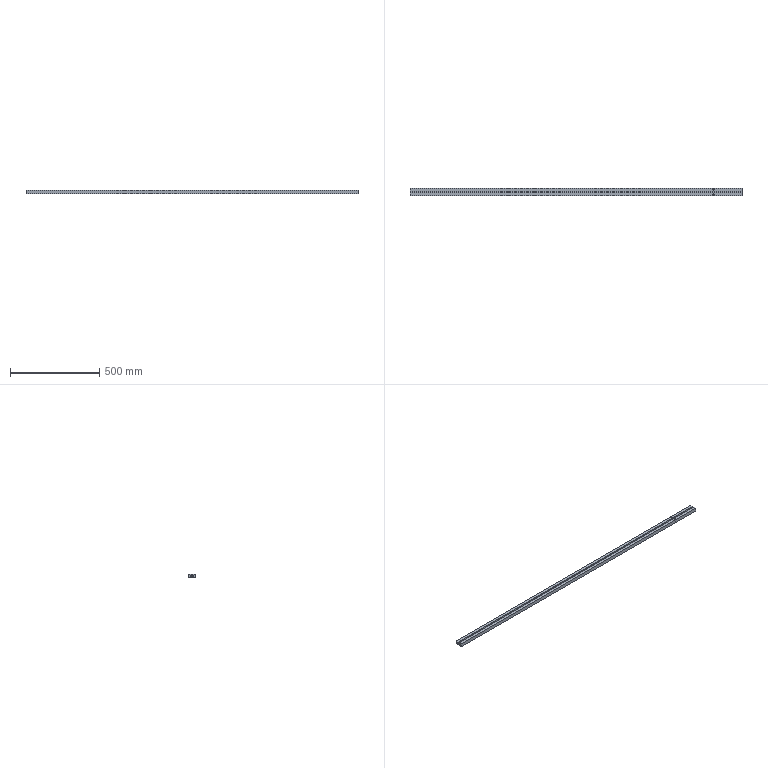Part | STEP file | DAOLIECHAO_1-2 | 1 solid | 28 faces | box 1861 x 40 x 20 mm | volume 1235153 mm3 | plane 20 | cylinder 8 | commonest cylinder face diameters 4.5 x4 8 x4
STEP:
#1=CARTESIAN_POINT('',(-377.75,-14.,-10.));
#2=VERTEX_POINT('',#1);
#3=CARTESIAN_POINT('',(-382.25,-14.,-10.));
#4=VERTEX_POINT('',#3);
#5=CARTESIAN_POINT('',(-380.,-14.,-10.));
#6=DIRECTION('',(0.,0.,-1.));
#7=DIRECTION('',(1.,0.,0.));
#8=AXIS2_PLACEMENT_3D('',#5,#6,#7);
#9=CIRCLE('',#8,2.25);
#10=EDGE_CURVE('',#2,#4,#9,.T.);
#11=ORIENTED_EDGE('',*,*,#10,.T.);
#12=CARTESIAN_POINT('',(-382.25,-14.,0.));
#13=VERTEX_POINT('',#12);
#14=CARTESIAN_POINT('',(-382.25,-14.,10.));
#15=DIRECTION('',(0.,0.,1.));
#16=VECTOR('',#15,1000.);
#17=LINE('',#14,#16);
#18=EDGE_CURVE('',#4,#13,#17,.T.);
#19=ORIENTED_EDGE('',*,*,#18,.T.);
#20=CARTESIAN_POINT('',(-377.75,-14.,0.));
#21=VERTEX_POINT('',#20);
#22=CARTESIAN_POINT('',(-380.,-14.,0.));
#23=DIRECTION('',(0.,0.,-1.));
#24=DIRECTION('',(1.,0.,0.));
#25=AXIS2_PLACEMENT_3D('',#22,#23,#24);
#26=CIRCLE('',#25,2.25);
#27=EDGE_CURVE('',#21,#13,#26,.T.);
#28=ORIENTED_EDGE('',*,*,#27,.F.);
#29=CARTESIAN_POINT('',(-377.75,-14.,10.));
#30=DIRECTION('',(0.,0.,1.));
#31=VECTOR('',#30,1000.);
#32=LINE('',#29,#31);
#33=EDGE_CURVE('',#2,#21,#32,.T.);
#34=ORIENTED_EDGE('',*,*,#33,.F.);
#35=EDGE_LOOP('',(#11,#19,#28,#34));
#36=FACE_OUTER_BOUND('',#35,.T.);
#37=CARTESIAN_POINT('',(-380.,-14.,10.));
#38=DIRECTION('',(0.,0.,1.));
#39=DIRECTION('',(1.,0.,0.));
#40=AXIS2_PLACEMENT_3D('',#37,#38,#39);
#41=CYLINDRICAL_SURFACE('',#40,2.25);
#42=ADVANCED_FACE('',(#36),#41,.F.);
#43=CARTESIAN_POINT('',(-377.75,14.,-10.));
#44=VERTEX_POINT('',#43);
#45=CARTESIAN_POINT('',(-382.25,14.,-10.));
#46=VERTEX_POINT('',#45);
#47=CARTESIAN_POINT('',(-380.,14.,-10.));
#48=DIRECTION('',(0.,0.,-1.));
#49=DIRECTION('',(1.,0.,0.));
#50=AXIS2_PLACEMENT_3D('',#47,#48,#49);
#51=CIRCLE('',#50,2.25);
#52=EDGE_CURVE('',#44,#46,#51,.T.);
#53=ORIENTED_EDGE('',*,*,#52,.T.);
#54=CARTESIAN_POINT('',(-382.25,14.,0.));
#55=VERTEX_POINT('',#54);
#56=CARTESIAN_POINT('',(-382.25,14.,10.));
#57=DIRECTION('',(0.,0.,1.));
#58=VECTOR('',#57,1000.);
#59=LINE('',#56,#58);
#60=EDGE_CURVE('',#46,#55,#59,.T.);
#61=ORIENTED_EDGE('',*,*,#60,.T.);
#62=CARTESIAN_POINT('',(-377.75,14.,0.));
#63=VERTEX_POINT('',#62);
#64=CARTESIAN_POINT('',(-380.,14.,0.));
#65=DIRECTION('',(0.,0.,-1.));
#66=DIRECTION('',(1.,0.,0.));
#67=AXIS2_PLACEMENT_3D('',#64,#65,#66);
#68=CIRCLE('',#67,2.25);
#69=EDGE_CURVE('',#63,#55,#68,.T.);
#70=ORIENTED_EDGE('',*,*,#69,.F.);
#71=CARTESIAN_POINT('',(-377.75,14.,10.));
#72=DIRECTION('',(0.,0.,1.));
#73=VECTOR('',#72,1000.);
#74=LINE('',#71,#73);
#75=EDGE_CURVE('',#44,#63,#74,.T.);
#76=ORIENTED_EDGE('',*,*,#75,.F.);
#77=EDGE_LOOP('',(#53,#61,#70,#76));
#78=FACE_OUTER_BOUND('',#77,.T.);
#79=CARTESIAN_POINT('',(-380.,14.,10.));
#80=DIRECTION('',(0.,0.,1.));
#81=DIRECTION('',(1.,0.,0.));
#82=AXIS2_PLACEMENT_3D('',#79,#80,#81);
#83=CYLINDRICAL_SURFACE('',#82,2.25);
#84=ADVANCED_FACE('',(#78),#83,.F.);
#85=CARTESIAN_POINT('',(-376.,-14.,0.));
#86=VERTEX_POINT('',#85);
#87=CARTESIAN_POINT('',(-384.,-14.,0.));
#88=VERTEX_POINT('',#87);
#89=CARTESIAN_POINT('',(-380.,-14.,0.));
#90=DIRECTION('',(0.,0.,-1.));
#91=DIRECTION('',(1.,0.,0.));
#92=AXIS2_PLACEMENT_3D('',#89,#90,#91);
#93=CIRCLE('',#92,4.);
#94=EDGE_CURVE('',#86,#88,#93,.T.);
#95=ORIENTED_EDGE('',*,*,#94,.T.);
#96=CARTESIAN_POINT('',(-384.,-14.,10.));
#97=VERTEX_POINT('',#96);
#98=CARTESIAN_POINT('',(-384.,-14.,10.));
#99=DIRECTION('',(0.,0.,1.));
#100=VECTOR('',#99,1000.);
#101=LINE('',#98,#100);
#102=EDGE_CURVE('',#88,#97,#101,.T.);
#103=ORIENTED_EDGE('',*,*,#102,.T.);
#104=CARTESIAN_POINT('',(-376.,-14.,10.));
#105=VERTEX_POINT('',#104);
#106=CARTESIAN_POINT('',(-380.,-14.,10.));
#107=DIRECTION('',(0.,0.,1.));
#108=DIRECTION('',(1.,0.,0.));
#109=AXIS2_PLACEMENT_3D('',#106,#107,#108);
#110=CIRCLE('',#109,4.);
#111=EDGE_CURVE('',#97,#105,#110,.T.);
#112=ORIENTED_EDGE('',*,*,#111,.T.);
#113=CARTESIAN_POINT('',(-376.,-14.,10.));
#114=DIRECTION('',(0.,0.,1.));
#115=VECTOR('',#114,1000.);
#116=LINE('',#113,#115);
#117=EDGE_CURVE('',#86,#105,#116,.T.);
#118=ORIENTED_EDGE('',*,*,#117,.F.);
#119=EDGE_LOOP('',(#95,#103,#112,#118));
#120=FACE_OUTER_BOUND('',#119,.T.);
#121=CARTESIAN_POINT('',(-380.,-14.,10.));
#122=DIRECTION('',(0.,0.,1.));
#123=DIRECTION('',(1.,0.,0.));
#124=AXIS2_PLACEMENT_3D('',#121,#122,#123);
#125=CYLINDRICAL_SURFACE('',#124,4.);
#126=ADVANCED_FACE('',(#120),#125,.F.);
#127=CARTESIAN_POINT('',(-376.,14.,0.));
#128=VERTEX_POINT('',#127);
#129=CARTESIAN_POINT('',(-384.,14.,0.));
#130=VERTEX_POINT('',#129);
#131=CARTESIAN_POINT('',(-380.,14.,0.));
#132=DIRECTION('',(0.,0.,-1.));
#133=DIRECTION('',(1.,0.,0.));
#134=AXIS2_PLACEMENT_3D('',#131,#132,#133);
#135=CIRCLE('',#134,4.);
#136=EDGE_CURVE('',#128,#130,#135,.T.);
#137=ORIENTED_EDGE('',*,*,#136,.T.);
#138=CARTESIAN_POINT('',(-384.,14.,10.));
#139=VERTEX_POINT('',#138);
#140=CARTESIAN_POINT('',(-384.,14.,10.));
#141=DIRECTION('',(0.,0.,1.));
#142=VECTOR('',#141,1000.);
#143=LINE('',#140,#142);
#144=EDGE_CURVE('',#130,#139,#143,.T.);
#145=ORIENTED_EDGE('',*,*,#144,.T.);
#146=CARTESIAN_POINT('',(-376.,14.,10.));
#147=VERTEX_POINT('',#146);
#148=CARTESIAN_POINT('',(-380.,14.,10.));
#149=DIRECTION('',(0.,0.,1.));
#150=DIRECTION('',(1.,0.,0.));
#151=AXIS2_PLACEMENT_3D('',#148,#149,#150);
#152=CIRCLE('',#151,4.);
#153=EDGE_CURVE('',#139,#147,#152,.T.);
#154=ORIENTED_EDGE('',*,*,#153,.T.);
#155=CARTESIAN_POINT('',(-376.,14.,10.));
#156=DIRECTION('',(0.,0.,1.));
#157=VECTOR('',#156,1000.);
#158=LINE('',#155,#157);
#159=EDGE_CURVE('',#128,#147,#158,.T.);
#160=ORIENTED_EDGE('',*,*,#159,.F.);
#161=EDGE_LOOP('',(#137,#145,#154,#160));
#162=FACE_OUTER_BOUND('',#161,.T.);
#163=CARTESIAN_POINT('',(-380.,14.,10.));
#164=DIRECTION('',(0.,0.,1.));
#165=DIRECTION('',(1.,0.,0.));
#166=AXIS2_PLACEMENT_3D('',#163,#164,#165);
#167=CYLINDRICAL_SURFACE('',#166,4.);
#168=ADVANCED_FACE('',(#162),#167,.F.);
#169=ORIENTED_EDGE('',*,*,#10,.F.);
#170=CARTESIAN_POINT('',(-380.,-14.,-10.));
#171=DIRECTION('',(0.,0.,-1.));
#172=DIRECTION('',(1.,0.,0.));
#173=AXIS2_PLACEMENT_3D('',#170,#171,#172);
#174=CIRCLE('',#173,2.25);
#175=EDGE_CURVE('',#4,#2,#174,.T.);
#176=ORIENTED_EDGE('',*,*,#175,.F.);
#177=EDGE_LOOP('',(#169,#176));
#178=FACE_BOUND('',#177,.T.);
#179=ORIENTED_EDGE('',*,*,#52,.F.);
#180=CARTESIAN_POINT('',(-380.,14.,-10.));
#181=DIRECTION('',(0.,0.,-1.));
#182=DIRECTION('',(1.,0.,0.));
#183=AXIS2_PLACEMENT_3D('',#180,#181,#182);
#184=CIRCLE('',#183,2.25);
#185=EDGE_CURVE('',#46,#44,#184,.T.);
#186=ORIENTED_EDGE('',*,*,#185,.F.);
#187=EDGE_LOOP('',(#179,#186));
#188=FACE_BOUND('',#187,.T.);
#189=CARTESIAN_POINT('',(-2082.,-20.,-10.));
#190=VERTEX_POINT('',#189);
#191=CARTESIAN_POINT('',(-220.621,-20.,-10.));
#192=VERTEX_POINT('',#191);
#193=CARTESIAN_POINT('',(400.,-20.,-10.));
#194=DIRECTION('',(1.,0.,0.));
#195=VECTOR('',#194,1000.);
#196=LINE('',#193,#195);
#197=EDGE_CURVE('',#190,#192,#196,.T.);
#198=ORIENTED_EDGE('',*,*,#197,.F.);
#199=CARTESIAN_POINT('',(-2082.,20.,-10.));
#200=VERTEX_POINT('',#199);
#201=CARTESIAN_POINT('',(-2082.,-20.,-10.));
#202=DIRECTION('',(0.,1.,0.));
#203=VECTOR('',#202,1000.);
#204=LINE('',#201,#203);
#205=EDGE_CURVE('',#190,#200,#204,.T.);
#206=ORIENTED_EDGE('',*,*,#205,.T.);
#207=CARTESIAN_POINT('',(-220.621,20.,-10.));
#208=VERTEX_POINT('',#207);
#209=CARTESIAN_POINT('',(400.,20.,-10.));
#210=DIRECTION('',(-1.,0.,0.));
#211=VECTOR('',#210,1000.);
#212=LINE('',#209,#211);
#213=EDGE_CURVE('',#208,#200,#212,.T.);
#214=ORIENTED_EDGE('',*,*,#213,.F.);
#215=CARTESIAN_POINT('',(-220.621,-20.,-10.));
#216=DIRECTION('',(0.,1.,0.));
#217=VECTOR('',#216,1000.);
#218=LINE('',#215,#217);
#219=EDGE_CURVE('',#192,#208,#218,.T.);
#220=ORIENTED_EDGE('',*,*,#219,.F.);
#221=EDGE_LOOP('',(#198,#206,#214,#220));
#222=FACE_OUTER_BOUND('',#221,.T.);
#223=CARTESIAN_POINT('',(400.,-20.,-10.));
#224=DIRECTION('',(0.,0.,1.));
#225=DIRECTION('',(1.,0.,0.));
#226=AXIS2_PLACEMENT_3D('',#223,#224,#225);
#227=PLANE('',#226);
#228=ADVANCED_FACE('',(#178,#188,#222),#227,.F.);
#229=ORIENTED_EDGE('',*,*,#18,.F.);
#230=ORIENTED_EDGE('',*,*,#175,.T.);
#231=ORIENTED_EDGE('',*,*,#33,.T.);
#232=CARTESIAN_POINT('',(-380.,-14.,0.));
#233=DIRECTION('',(0.,0.,-1.));
#234=DIRECTION('',(1.,0.,0.));
#235=AXIS2_PLACEMENT_3D('',#232,#233,#234);
#236=CIRCLE('',#235,2.25);
#237=EDGE_CURVE('',#13,#21,#236,.T.);
#238=ORIENTED_EDGE('',*,*,#237,.F.);
#239=EDGE_LOOP('',(#229,#230,#231,#238));
#240=FACE_OUTER_BOUND('',#239,.T.);
#241=CARTESIAN_POINT('',(-380.,-14.,10.));
#242=DIRECTION('',(0.,0.,1.));
#243=DIRECTION('',(1.,0.,0.));
#244=AXIS2_PLACEMENT_3D('',#241,#242,#243);
#245=CYLINDRICAL_SURFACE('',#244,2.25);
#246=ADVANCED_FACE('',(#240),#245,.F.);
#247=ORIENTED_EDGE('',*,*,#60,.F.);
#248=ORIENTED_EDGE('',*,*,#185,.T.);
#249=ORIENTED_EDGE('',*,*,#75,.T.);
#250=CARTESIAN_POINT('',(-380.,14.,0.));
#251=DIRECTION('',(0.,0.,-1.));
#252=DIRECTION('',(1.,0.,0.));
#253=AXIS2_PLACEMENT_3D('',#250,#251,#252);
#254=CIRCLE('',#253,2.25);
#255=EDGE_CURVE('',#55,#63,#254,.T.);
#256=ORIENTED_EDGE('',*,*,#255,.F.);
#257=EDGE_LOOP('',(#247,#248,#249,#256));
#258=FACE_OUTER_BOUND('',#257,.T.);
#259=CARTESIAN_POINT('',(-380.,14.,10.));
#260=DIRECTION('',(0.,0.,1.));
#261=DIRECTION('',(1.,0.,0.));
#262=AXIS2_PLACEMENT_3D('',#259,#260,#261);
#263=CYLINDRICAL_SURFACE('',#262,2.25);
#264=ADVANCED_FACE('',(#258),#263,.F.);
#265=ORIENTED_EDGE('',*,*,#213,.T.);
#266=CARTESIAN_POINT('',(-2082.,20.,10.));
#267=VERTEX_POINT('',#266);
#268=CARTESIAN_POINT('',(-2082.,20.,-10.));
#269=DIRECTION('',(0.,0.,1.));
#270=VECTOR('',#269,1000.);
#271=LINE('',#268,#270);
#272=EDGE_CURVE('',#200,#267,#271,.T.);
#273=ORIENTED_EDGE('',*,*,#272,.T.);
#274=CARTESIAN_POINT('',(-220.621,20.,10.));
#275=VERTEX_POINT('',#274);
#276=CARTESIAN_POINT('',(400.,20.,10.));
#277=DIRECTION('',(-1.,0.,0.));
#278=VECTOR('',#277,1000.);
#279=LINE('',#276,#278);
#280=EDGE_CURVE('',#275,#267,#279,.T.);
#281=ORIENTED_EDGE('',*,*,#280,.F.);
#282=CARTESIAN_POINT('',(-220.621,20.,-10.));
#283=DIRECTION('',(0.,0.,-1.));
#284=VECTOR('',#283,1000.);
#285=LINE('',#282,#284);
#286=EDGE_CURVE('',#275,#208,#285,.T.);
#287=ORIENTED_EDGE('',*,*,#286,.T.);
#288=EDGE_LOOP('',(#265,#273,#281,#287));
#289=FACE_OUTER_BOUND('',#288,.T.);
#290=CARTESIAN_POINT('',(400.,20.,-10.));
#291=DIRECTION('',(0.,-1.,0.));
#292=DIRECTION('',(0.,0.,-1.));
#293=AXIS2_PLACEMENT_3D('',#290,#291,#292);
#294=PLANE('',#293);
#295=ADVANCED_FACE('',(#289),#294,.F.);
#296=CARTESIAN_POINT('',(-2082.,-20.,10.));
#297=VERTEX_POINT('',#296);
#298=CARTESIAN_POINT('',(-220.621,-20.,10.));
#299=VERTEX_POINT('',#298);
#300=CARTESIAN_POINT('',(400.,-20.,10.));
#301=DIRECTION('',(1.,0.,0.));
#302=VECTOR('',#301,1000.);
#303=LINE('',#300,#302);
#304=EDGE_CURVE('',#297,#299,#303,.T.);
#305=ORIENTED_EDGE('',*,*,#304,.F.);
#306=CARTESIAN_POINT('',(-2082.,-20.,-10.));
#307=DIRECTION('',(0.,0.,-1.));
#308=VECTOR('',#307,1000.);
#309=LINE('',#306,#308);
#310=EDGE_CURVE('',#297,#190,#309,.T.);
#311=ORIENTED_EDGE('',*,*,#310,.T.);
#312=ORIENTED_EDGE('',*,*,#197,.T.);
#313=CARTESIAN_POINT('',(-220.621,-20.,10.));
#314=DIRECTION('',(0.,0.,-1.));
#315=VECTOR('',#314,1000.);
#316=LINE('',#313,#315);
#317=EDGE_CURVE('',#299,#192,#316,.T.);
#318=ORIENTED_EDGE('',*,*,#317,.F.);
#319=EDGE_LOOP('',(#305,#311,#312,#318));
#320=FACE_OUTER_BOUND('',#319,.T.);
#321=CARTESIAN_POINT('',(400.,-20.,-10.));
#322=DIRECTION('',(0.,1.,0.));
#323=DIRECTION('',(0.,0.,1.));
#324=AXIS2_PLACEMENT_3D('',#321,#322,#323);
#325=PLANE('',#324);
#326=ADVANCED_FACE('',(#320),#325,.F.);
#327=ORIENTED_EDGE('',*,*,#27,.T.);
#328=ORIENTED_EDGE('',*,*,#237,.T.);
#329=EDGE_LOOP('',(#327,#328));
#330=FACE_BOUND('',#329,.T.);
#331=ORIENTED_EDGE('',*,*,#94,.F.);
#332=CARTESIAN_POINT('',(-380.,-14.,0.));
#333=DIRECTION('',(0.,0.,-1.));
#334=DIRECTION('',(1.,0.,0.));
#335=AXIS2_PLACEMENT_3D('',#332,#333,#334);
#336=CIRCLE('',#335,4.);
#337=EDGE_CURVE('',#88,#86,#336,.T.);
#338=ORIENTED_EDGE('',*,*,#337,.F.);
#339=EDGE_LOOP('',(#331,#338));
#340=FACE_OUTER_BOUND('',#339,.T.);
#341=CARTESIAN_POINT('',(-377.75,-14.,0.));
#342=DIRECTION('',(0.,0.,-1.));
#343=DIRECTION('',(-1.,0.,0.));
#344=AXIS2_PLACEMENT_3D('',#341,#342,#343);
#345=PLANE('',#344);
#346=ADVANCED_FACE('',(#330,#340),#345,.F.);
#347=ORIENTED_EDGE('',*,*,#69,.T.);
#348=ORIENTED_EDGE('',*,*,#255,.T.);
#349=EDGE_LOOP('',(#347,#348));
#350=FACE_BOUND('',#349,.T.);
#351=ORIENTED_EDGE('',*,*,#136,.F.);
#352=CARTESIAN_POINT('',(-380.,14.,0.));
#353=DIRECTION('',(0.,0.,-1.));
#354=DIRECTION('',(1.,0.,0.));
#355=AXIS2_PLACEMENT_3D('',#352,#353,#354);
#356=CIRCLE('',#355,4.);
#357=EDGE_CURVE('',#130,#128,#356,.T.);
#358=ORIENTED_EDGE('',*,*,#357,.F.);
#359=EDGE_LOOP('',(#351,#358));
#360=FACE_OUTER_BOUND('',#359,.T.);
#361=CARTESIAN_POINT('',(-377.75,14.,0.));
#362=DIRECTION('',(0.,0.,-1.));
#363=DIRECTION('',(-1.,0.,0.));
#364=AXIS2_PLACEMENT_3D('',#361,#362,#363);
#365=PLANE('',#364);
#366=ADVANCED_FACE('',(#350,#360),#365,.F.);
#367=CARTESIAN_POINT('',(-380.,14.,10.));
#368=DIRECTION('',(0.,0.,1.));
#369=DIRECTION('',(1.,0.,0.));
#370=AXIS2_PLACEMENT_3D('',#367,#368,#369);
#371=CIRCLE('',#370,4.);
#372=EDGE_CURVE('',#147,#139,#371,.T.);
#373=ORIENTED_EDGE('',*,*,#372,.F.);
#374=ORIENTED_EDGE('',*,*,#153,.F.);
#375=EDGE_LOOP('',(#373,#374));
#376=FACE_BOUND('',#375,.T.);
#377=ORIENTED_EDGE('',*,*,#280,.T.);
#378=CARTESIAN_POINT('',(-2082.,4.2,10.));
#379=VERTEX_POINT('',#378);
#380=CARTESIAN_POINT('',(-2082.,-22.,10.));
#381=DIRECTION('',(0.,1.,0.));
#382=VECTOR('',#381,1000.);
#383=LINE('',#380,#382);
#384=EDGE_CURVE('',#379,#267,#383,.T.);
#385=ORIENTED_EDGE('',*,*,#384,.F.);
#386=CARTESIAN_POINT('',(-220.621,4.2,10.));
#387=VERTEX_POINT('',#386);
#388=CARTESIAN_POINT('',(400.,4.2,10.));
#389=DIRECTION('',(-1.,0.,0.));
#390=VECTOR('',#389,1000.);
#391=LINE('',#388,#390);
#392=EDGE_CURVE('',#387,#379,#391,.T.);
#393=ORIENTED_EDGE('',*,*,#392,.F.);
#394=CARTESIAN_POINT('',(-220.621,-20.,10.));
#395=DIRECTION('',(0.,1.,0.));
#396=VECTOR('',#395,1000.);
#397=LINE('',#394,#396);
#398=EDGE_CURVE('',#387,#275,#397,.T.);
#399=ORIENTED_EDGE('',*,*,#398,.T.);
#400=EDGE_LOOP('',(#377,#385,#393,#399));
#401=FACE_OUTER_BOUND('',#400,.T.);
#402=CARTESIAN_POINT('',(400.,-20.,10.));
#403=DIRECTION('',(0.,0.,-1.));
#404=DIRECTION('',(-1.,0.,0.));
#405=AXIS2_PLACEMENT_3D('',#402,#403,#404);
#406=PLANE('',#405);
#407=ADVANCED_FACE('',(#376,#401),#406,.F.);
#408=ORIENTED_EDGE('',*,*,#392,.T.);
#409=CARTESIAN_POINT('',(-2082.,4.2,2.6));
#410=VERTEX_POINT('',#409);
#411=CARTESIAN_POINT('',(-2082.,4.2,10.));
#412=DIRECTION('',(0.,0.,-1.));
#413=VECTOR('',#412,1000.);
#414=LINE('',#411,#413);
#415=EDGE_CURVE('',#379,#410,#414,.T.);
#416=ORIENTED_EDGE('',*,*,#415,.T.);
#417=CARTESIAN_POINT('',(-220.621,4.2,2.6));
#418=VERTEX_POINT('',#417);
#419=CARTESIAN_POINT('',(-400.,4.2,2.6));
#420=DIRECTION('',(-1.,0.,0.));
#421=VECTOR('',#420,1000.);
#422=LINE('',#419,#421);
#423=EDGE_CURVE('',#418,#410,#422,.T.);
#424=ORIENTED_EDGE('',*,*,#423,.F.);
#425=CARTESIAN_POINT('',(-220.621,4.2,10.));
#426=DIRECTION('',(0.,0.,1.));
#427=VECTOR('',#426,1000.);
#428=LINE('',#425,#427);
#429=EDGE_CURVE('',#418,#387,#428,.T.);
#430=ORIENTED_EDGE('',*,*,#429,.T.);
#431=EDGE_LOOP('',(#408,#416,#424,#430));
#432=FACE_OUTER_BOUND('',#431,.T.);
#433=CARTESIAN_POINT('',(-400.,4.2,10.));
#434=DIRECTION('',(0.,1.,0.));
#435=DIRECTION('',(0.,0.,1.));
#436=AXIS2_PLACEMENT_3D('',#433,#434,#435);
#437=PLANE('',#436);
#438=ADVANCED_FACE('',(#432),#437,.F.);
#439=CARTESIAN_POINT('',(-380.,-14.,10.));
#440=DIRECTION('',(0.,0.,1.));
#441=DIRECTION('',(1.,0.,0.));
#442=AXIS2_PLACEMENT_3D('',#439,#440,#441);
#443=CIRCLE('',#442,4.);
#444=EDGE_CURVE('',#105,#97,#443,.T.);
#445=ORIENTED_EDGE('',*,*,#444,.F.);
#446=ORIENTED_EDGE('',*,*,#111,.F.);
#447=EDGE_LOOP('',(#445,#446));
#448=FACE_BOUND('',#447,.T.);
#449=CARTESIAN_POINT('',(-2082.,-4.2,10.));
#450=VERTEX_POINT('',#449);
#451=CARTESIAN_POINT('',(-220.621,-4.2,10.));
#452=VERTEX_POINT('',#451);
#453=CARTESIAN_POINT('',(400.,-4.2,10.));
#454=DIRECTION('',(1.,0.,0.));
#455=VECTOR('',#454,1000.);
#456=LINE('',#453,#455);
#457=EDGE_CURVE('',#450,#452,#456,.T.);
#458=ORIENTED_EDGE('',*,*,#457,.F.);
#459=CARTESIAN_POINT('',(-2082.,-22.,10.));
#460=DIRECTION('',(0.,1.,0.));
#461=VECTOR('',#460,1000.);
#462=LINE('',#459,#461);
#463=EDGE_CURVE('',#297,#450,#462,.T.);
#464=ORIENTED_EDGE('',*,*,#463,.F.);
#465=ORIENTED_EDGE('',*,*,#304,.T.);
#466=CARTESIAN_POINT('',(-220.621,-20.,10.));
#467=DIRECTION('',(0.,1.,0.));
#468=VECTOR('',#467,1000.);
#469=LINE('',#466,#468);
#470=EDGE_CURVE('',#299,#452,#469,.T.);
#471=ORIENTED_EDGE('',*,*,#470,.T.);
#472=EDGE_LOOP('',(#458,#464,#465,#471));
#473=FACE_OUTER_BOUND('',#472,.T.);
#474=CARTESIAN_POINT('',(400.,-20.,10.));
#475=DIRECTION('',(0.,0.,-1.));
#476=DIRECTION('',(-1.,0.,0.));
#477=AXIS2_PLACEMENT_3D('',#474,#475,#476);
#478=PLANE('',#477);
#479=ADVANCED_FACE('',(#448,#473),#478,.F.);
#480=CARTESIAN_POINT('',(-2082.,-4.2,2.6));
#481=VERTEX_POINT('',#480);
#482=CARTESIAN_POINT('',(-220.621,-4.2,2.6));
#483=VERTEX_POINT('',#482);
#484=CARTESIAN_POINT('',(-400.,-4.2,2.6));
#485=DIRECTION('',(1.,0.,0.));
#486=VECTOR('',#485,1000.);
#487=LINE('',#484,#486);
#488=EDGE_CURVE('',#481,#483,#487,.T.);
#489=ORIENTED_EDGE('',*,*,#488,.F.);
#490=CARTESIAN_POINT('',(-2082.,-4.2,2.6));
#491=DIRECTION('',(0.,0.,1.));
#492=VECTOR('',#491,1000.);
#493=LINE('',#490,#492);
#494=EDGE_CURVE('',#481,#450,#493,.T.);
#495=ORIENTED_EDGE('',*,*,#494,.T.);
#496=ORIENTED_EDGE('',*,*,#457,.T.);
#497=CARTESIAN_POINT('',(-220.621,-4.2,2.6));
#498=DIRECTION('',(0.,0.,-1.));
#499=VECTOR('',#498,1000.);
#500=LINE('',#497,#499);
#501=EDGE_CURVE('',#452,#483,#500,.T.);
#502=ORIENTED_EDGE('',*,*,#501,.T.);
#503=EDGE_LOOP('',(#489,#495,#496,#502));
#504=FACE_OUTER_BOUND('',#503,.T.);
#505=CARTESIAN_POINT('',(-400.,-4.2,2.6));
#506=DIRECTION('',(0.,-1.,0.));
#507=DIRECTION('',(0.,0.,-1.));
#508=AXIS2_PLACEMENT_3D('',#505,#506,#507);
#509=PLANE('',#508);
#510=ADVANCED_FACE('',(#504),#509,.F.);
#511=CARTESIAN_POINT('',(-2082.,-6.6,2.6));
#512=VERTEX_POINT('',#511);
#513=CARTESIAN_POINT('',(-220.621,-6.6,2.6));
#514=VERTEX_POINT('',#513);
#515=CARTESIAN_POINT('',(-400.,-6.6,2.6));
#516=DIRECTION('',(1.,0.,0.));
#517=VECTOR('',#516,1000.);
#518=LINE('',#515,#517);
#519=EDGE_CURVE('',#512,#514,#518,.T.);
#520=ORIENTED_EDGE('',*,*,#519,.F.);
#521=CARTESIAN_POINT('',(-2082.,-6.6,2.6));
#522=DIRECTION('',(0.,1.,0.));
#523=VECTOR('',#522,1000.);
#524=LINE('',#521,#523);
#525=EDGE_CURVE('',#512,#481,#524,.T.);
#526=ORIENTED_EDGE('',*,*,#525,.T.);
#527=ORIENTED_EDGE('',*,*,#488,.T.);
#528=CARTESIAN_POINT('',(-220.621,-6.6,2.6));
#529=DIRECTION('',(0.,-1.,0.));
#530=VECTOR('',#529,1000.);
#531=LINE('',#528,#530);
#532=EDGE_CURVE('',#483,#514,#531,.T.);
#533=ORIENTED_EDGE('',*,*,#532,.T.);
#534=EDGE_LOOP('',(#520,#526,#527,#533));
#535=FACE_OUTER_BOUND('',#534,.T.);
#536=CARTESIAN_POINT('',(-400.,-6.6,2.6));
#537=DIRECTION('',(0.,0.,1.));
#538=DIRECTION('',(1.,0.,0.));
#539=AXIS2_PLACEMENT_3D('',#536,#537,#538);
#540=PLANE('',#539);
#541=ADVANCED_FACE('',(#535),#540,.F.);
#542=CARTESIAN_POINT('',(-2082.,-6.6,-1.7));
#543=VERTEX_POINT('',#542);
#544=CARTESIAN_POINT('',(-220.621,-6.6,-1.7));
#545=VERTEX_POINT('',#544);
#546=CARTESIAN_POINT('',(-400.,-6.6,-1.7));
#547=DIRECTION('',(1.,0.,0.));
#548=VECTOR('',#547,1000.);
#549=LINE('',#546,#548);
#550=EDGE_CURVE('',#543,#545,#549,.T.);
#551=ORIENTED_EDGE('',*,*,#550,.F.);
#552=CARTESIAN_POINT('',(-2082.,-6.6,-1.7));
#553=DIRECTION('',(0.,0.,1.));
#554=VECTOR('',#553,1000.);
#555=LINE('',#552,#554);
#556=EDGE_CURVE('',#543,#512,#555,.T.);
#557=ORIENTED_EDGE('',*,*,#556,.T.);
#558=ORIENTED_EDGE('',*,*,#519,.T.);
#559=CARTESIAN_POINT('',(-220.621,-6.6,-1.7));
#560=DIRECTION('',(0.,0.,-1.));
#561=VECTOR('',#560,1000.);
#562=LINE('',#559,#561);
#563=EDGE_CURVE('',#514,#545,#562,.T.);
#564=ORIENTED_EDGE('',*,*,#563,.T.);
#565=EDGE_LOOP('',(#551,#557,#558,#564));
#566=FACE_OUTER_BOUND('',#565,.T.);
#567=CARTESIAN_POINT('',(-400.,-6.6,-1.7));
#568=DIRECTION('',(0.,-1.,0.));
#569=DIRECTION('',(0.,0.,-1.));
#570=AXIS2_PLACEMENT_3D('',#567,#568,#569);
#571=PLANE('',#570);
#572=ADVANCED_FACE('',(#566),#571,.F.);
#573=CARTESIAN_POINT('',(-2082.,-4.2,-1.7));
#574=VERTEX_POINT('',#573);
#575=CARTESIAN_POINT('',(-220.621,-4.2,-1.7));
#576=VERTEX_POINT('',#575);
#577=CARTESIAN_POINT('',(-400.,-4.2,-1.7));
#578=DIRECTION('',(1.,0.,0.));
#579=VECTOR('',#578,1000.);
#580=LINE('',#577,#579);
#581=EDGE_CURVE('',#574,#576,#580,.T.);
#582=ORIENTED_EDGE('',*,*,#581,.F.);
#583=CARTESIAN_POINT('',(-2082.,-4.2,-1.7));
#584=DIRECTION('',(0.,-1.,0.));
#585=VECTOR('',#584,1000.);
#586=LINE('',#583,#585);
#587=EDGE_CURVE('',#574,#543,#586,.T.);
#588=ORIENTED_EDGE('',*,*,#587,.T.);
#589=ORIENTED_EDGE('',*,*,#550,.T.);
#590=CARTESIAN_POINT('',(-220.621,-4.2,-1.7));
#591=DIRECTION('',(0.,1.,0.));
#592=VECTOR('',#591,1000.);
#593=LINE('',#590,#592);
#594=EDGE_CURVE('',#545,#576,#593,.T.);
#595=ORIENTED_EDGE('',*,*,#594,.T.);
#596=EDGE_LOOP('',(#582,#588,#589,#595));
#597=FACE_OUTER_BOUND('',#596,.T.);
#598=CARTESIAN_POINT('',(-400.,-4.2,-1.7));
#599=DIRECTION('',(0.,0.,-1.));
#600=DIRECTION('',(-1.,0.,0.));
#601=AXIS2_PLACEMENT_3D('',#598,#599,#600);
#602=PLANE('',#601);
#603=ADVANCED_FACE('',(#597),#602,.F.);
#604=CARTESIAN_POINT('',(-2082.,-4.2,-3.7));
#605=VERTEX_POINT('',#604);
#606=CARTESIAN_POINT('',(-220.621,-4.2,-3.7));
#607=VERTEX_POINT('',#606);
#608=CARTESIAN_POINT('',(-400.,-4.2,-3.7));
#609=DIRECTION('',(1.,0.,0.));
#610=VECTOR('',#609,1000.);
#611=LINE('',#608,#610);
#612=EDGE_CURVE('',#605,#607,#611,.T.);
#613=ORIENTED_EDGE('',*,*,#612,.F.);
#614=CARTESIAN_POINT('',(-2082.,-4.2,-3.7));
#615=DIRECTION('',(0.,0.,1.));
#616=VECTOR('',#615,1000.);
#617=LINE('',#614,#616);
#618=EDGE_CURVE('',#605,#574,#617,.T.);
#619=ORIENTED_EDGE('',*,*,#618,.T.);
#620=ORIENTED_EDGE('',*,*,#581,.T.);
#621=CARTESIAN_POINT('',(-220.621,-4.2,-3.7));
#622=DIRECTION('',(0.,0.,-1.));
#623=VECTOR('',#622,1000.);
#624=LINE('',#621,#623);
#625=EDGE_CURVE('',#576,#607,#624,.T.);
#626=ORIENTED_EDGE('',*,*,#625,.T.);
#627=EDGE_LOOP('',(#613,#619,#620,#626));
#628=FACE_OUTER_BOUND('',#627,.T.);
#629=CARTESIAN_POINT('',(-400.,-4.2,-3.7));
#630=DIRECTION('',(0.,-1.,0.));
#631=DIRECTION('',(0.,0.,-1.));
#632=AXIS2_PLACEMENT_3D('',#629,#630,#631);
#633=PLANE('',#632);
#634=ADVANCED_FACE('',(#628),#633,.F.);
#635=CARTESIAN_POINT('',(-2082.,4.2,-3.7));
#636=VERTEX_POINT('',#635);
#637=CARTESIAN_POINT('',(-220.621,4.2,-3.7));
#638=VERTEX_POINT('',#637);
#639=CARTESIAN_POINT('',(-400.,4.2,-3.7));
#640=DIRECTION('',(1.,0.,0.));
#641=VECTOR('',#640,1000.);
#642=LINE('',#639,#641);
#643=EDGE_CURVE('',#636,#638,#642,.T.);
#644=ORIENTED_EDGE('',*,*,#643,.F.);
#645=CARTESIAN_POINT('',(-2082.,4.2,-3.7));
#646=DIRECTION('',(0.,-1.,0.));
#647=VECTOR('',#646,1000.);
#648=LINE('',#645,#647);
#649=EDGE_CURVE('',#636,#605,#648,.T.);
#650=ORIENTED_EDGE('',*,*,#649,.T.);
#651=ORIENTED_EDGE('',*,*,#612,.T.);
#652=CARTESIAN_POINT('',(-220.621,4.2,-3.7));
#653=DIRECTION('',(0.,1.,0.));
#654=VECTOR('',#653,1000.);
#655=LINE('',#652,#654);
#656=EDGE_CURVE('',#607,#638,#655,.T.);
#657=ORIENTED_EDGE('',*,*,#656,.T.);
#658=EDGE_LOOP('',(#644,#650,#651,#657));
#659=FACE_OUTER_BOUND('',#658,.T.);
#660=CARTESIAN_POINT('',(-400.,4.2,-3.7));
#661=DIRECTION('',(0.,0.,-1.));
#662=DIRECTION('',(-1.,0.,0.));
#663=AXIS2_PLACEMENT_3D('',#660,#661,#662);
#664=PLANE('',#663);
#665=ADVANCED_FACE('',(#659),#664,.F.);
#666=CARTESIAN_POINT('',(-2082.,4.2,-1.7));
#667=VERTEX_POINT('',#666);
#668=CARTESIAN_POINT('',(-220.621,4.2,-1.7));
#669=VERTEX_POINT('',#668);
#670=CARTESIAN_POINT('',(-400.,4.2,-1.7));
#671=DIRECTION('',(1.,0.,0.));
#672=VECTOR('',#671,1000.);
#673=LINE('',#670,#672);
#674=EDGE_CURVE('',#667,#669,#673,.T.);
#675=ORIENTED_EDGE('',*,*,#674,.F.);
#676=CARTESIAN_POINT('',(-2082.,4.2,-1.7));
#677=DIRECTION('',(0.,0.,-1.));
#678=VECTOR('',#677,1000.);
#679=LINE('',#676,#678);
#680=EDGE_CURVE('',#667,#636,#679,.T.);
#681=ORIENTED_EDGE('',*,*,#680,.T.);
#682=ORIENTED_EDGE('',*,*,#643,.T.);
#683=CARTESIAN_POINT('',(-220.621,4.2,-1.7));
#684=DIRECTION('',(0.,0.,1.));
#685=VECTOR('',#684,1000.);
#686=LINE('',#683,#685);
#687=EDGE_CURVE('',#638,#669,#686,.T.);
#688=ORIENTED_EDGE('',*,*,#687,.T.);
#689=EDGE_LOOP('',(#675,#681,#682,#688));
#690=FACE_OUTER_BOUND('',#689,.T.);
#691=CARTESIAN_POINT('',(-400.,4.2,-1.7));
#692=DIRECTION('',(0.,1.,0.));
#693=DIRECTION('',(0.,0.,1.));
#694=AXIS2_PLACEMENT_3D('',#691,#692,#693);
#695=PLANE('',#694);
#696=ADVANCED_FACE('',(#690),#695,.F.);
#697=CARTESIAN_POINT('',(-2082.,6.6,-1.7));
#698=VERTEX_POINT('',#697);
#699=CARTESIAN_POINT('',(-220.621,6.6,-1.7));
#700=VERTEX_POINT('',#699);
#701=CARTESIAN_POINT('',(-400.,6.6,-1.7));
#702=DIRECTION('',(1.,0.,0.));
#703=VECTOR('',#702,1000.);
#704=LINE('',#701,#703);
#705=EDGE_CURVE('',#698,#700,#704,.T.);
#706=ORIENTED_EDGE('',*,*,#705,.F.);
#707=CARTESIAN_POINT('',(-2082.,6.6,-1.7));
#708=DIRECTION('',(0.,-1.,0.));
#709=VECTOR('',#708,1000.);
#710=LINE('',#707,#709);
#711=EDGE_CURVE('',#698,#667,#710,.T.);
#712=ORIENTED_EDGE('',*,*,#711,.T.);
#713=ORIENTED_EDGE('',*,*,#674,.T.);
#714=CARTESIAN_POINT('',(-220.621,6.6,-1.7));
#715=DIRECTION('',(0.,1.,0.));
#716=VECTOR('',#715,1000.);
#717=LINE('',#714,#716);
#718=EDGE_CURVE('',#669,#700,#717,.T.);
#719=ORIENTED_EDGE('',*,*,#718,.T.);
#720=EDGE_LOOP('',(#706,#712,#713,#719));
#721=FACE_OUTER_BOUND('',#720,.T.);
#722=CARTESIAN_POINT('',(-400.,6.6,-1.7));
#723=DIRECTION('',(0.,0.,-1.));
#724=DIRECTION('',(-1.,0.,0.));
#725=AXIS2_PLACEMENT_3D('',#722,#723,#724);
#726=PLANE('',#725);
#727=ADVANCED_FACE('',(#721),#726,.F.);
#728=CARTESIAN_POINT('',(-2082.,6.6,2.6));
#729=VERTEX_POINT('',#728);
#730=CARTESIAN_POINT('',(-220.621,6.6,2.6));
#731=VERTEX_POINT('',#730);
#732=CARTESIAN_POINT('',(-400.,6.6,2.6));
#733=DIRECTION('',(1.,0.,0.));
#734=VECTOR('',#733,1000.);
#735=LINE('',#732,#734);
#736=EDGE_CURVE('',#729,#731,#735,.T.);
#737=ORIENTED_EDGE('',*,*,#736,.F.);
#738=CARTESIAN_POINT('',(-2082.,6.6,2.6));
#739=DIRECTION('',(0.,0.,-1.));
#740=VECTOR('',#739,1000.);
#741=LINE('',#738,#740);
#742=EDGE_CURVE('',#729,#698,#741,.T.);
#743=ORIENTED_EDGE('',*,*,#742,.T.);
#744=ORIENTED_EDGE('',*,*,#705,.T.);
#745=CARTESIAN_POINT('',(-220.621,6.6,2.6));
#746=DIRECTION('',(0.,0.,1.));
#747=VECTOR('',#746,1000.);
#748=LINE('',#745,#747);
#749=EDGE_CURVE('',#700,#731,#748,.T.);
#750=ORIENTED_EDGE('',*,*,#749,.T.);
#751=EDGE_LOOP('',(#737,#743,#744,#750));
#752=FACE_OUTER_BOUND('',#751,.T.);
#753=CARTESIAN_POINT('',(-400.,6.6,2.6));
#754=DIRECTION('',(0.,1.,0.));
#755=DIRECTION('',(0.,0.,1.));
#756=AXIS2_PLACEMENT_3D('',#753,#754,#755);
#757=PLANE('',#756);
#758=ADVANCED_FACE('',(#752),#757,.F.);
#759=ORIENTED_EDGE('',*,*,#423,.T.);
#760=CARTESIAN_POINT('',(-2082.,4.2,2.6));
#761=DIRECTION('',(0.,1.,0.));
#762=VECTOR('',#761,1000.);
#763=LINE('',#760,#762);
#764=EDGE_CURVE('',#410,#729,#763,.T.);
#765=ORIENTED_EDGE('',*,*,#764,.T.);
#766=ORIENTED_EDGE('',*,*,#736,.T.);
#767=CARTESIAN_POINT('',(-220.621,4.2,2.6));
#768=DIRECTION('',(0.,-1.,0.));
#769=VECTOR('',#768,1000.);
#770=LINE('',#767,#769);
#771=EDGE_CURVE('',#731,#418,#770,.T.);
#772=ORIENTED_EDGE('',*,*,#771,.T.);
#773=EDGE_LOOP('',(#759,#765,#766,#772));
#774=FACE_OUTER_BOUND('',#773,.T.);
#775=CARTESIAN_POINT('',(-400.,4.2,2.6));
#776=DIRECTION('',(0.,0.,1.));
#777=DIRECTION('',(1.,0.,0.));
#778=AXIS2_PLACEMENT_3D('',#775,#776,#777);
#779=PLANE('',#778);
#780=ADVANCED_FACE('',(#774),#779,.F.);
#781=ORIENTED_EDGE('',*,*,#102,.F.);
#782=ORIENTED_EDGE('',*,*,#337,.T.);
#783=ORIENTED_EDGE('',*,*,#117,.T.);
#784=ORIENTED_EDGE('',*,*,#444,.T.);
#785=EDGE_LOOP('',(#781,#782,#783,#784));
#786=FACE_OUTER_BOUND('',#785,.T.);
#787=CARTESIAN_POINT('',(-380.,-14.,10.));
#788=DIRECTION('',(0.,0.,1.));
#789=DIRECTION('',(1.,0.,0.));
#790=AXIS2_PLACEMENT_3D('',#787,#788,#789);
#791=CYLINDRICAL_SURFACE('',#790,4.);
#792=ADVANCED_FACE('',(#786),#791,.F.);
#793=ORIENTED_EDGE('',*,*,#144,.F.);
#794=ORIENTED_EDGE('',*,*,#357,.T.);
#795=ORIENTED_EDGE('',*,*,#159,.T.);
#796=ORIENTED_EDGE('',*,*,#372,.T.);
#797=EDGE_LOOP('',(#793,#794,#795,#796));
#798=FACE_OUTER_BOUND('',#797,.T.);
#799=CARTESIAN_POINT('',(-380.,14.,10.));
#800=DIRECTION('',(0.,0.,1.));
#801=DIRECTION('',(1.,0.,0.));
#802=AXIS2_PLACEMENT_3D('',#799,#800,#801);
#803=CYLINDRICAL_SURFACE('',#802,4.);
#804=ADVANCED_FACE('',(#798),#803,.F.);
#805=ORIENTED_EDGE('',*,*,#470,.F.);
#806=ORIENTED_EDGE('',*,*,#317,.T.);
#807=ORIENTED_EDGE('',*,*,#219,.T.);
#808=ORIENTED_EDGE('',*,*,#286,.F.);
#809=ORIENTED_EDGE('',*,*,#398,.F.);
#810=ORIENTED_EDGE('',*,*,#429,.F.);
#811=ORIENTED_EDGE('',*,*,#771,.F.);
#812=ORIENTED_EDGE('',*,*,#749,.F.);
#813=ORIENTED_EDGE('',*,*,#718,.F.);
#814=ORIENTED_EDGE('',*,*,#687,.F.);
#815=ORIENTED_EDGE('',*,*,#656,.F.);
#816=ORIENTED_EDGE('',*,*,#625,.F.);
#817=ORIENTED_EDGE('',*,*,#594,.F.);
#818=ORIENTED_EDGE('',*,*,#563,.F.);
#819=ORIENTED_EDGE('',*,*,#532,.F.);
#820=ORIENTED_EDGE('',*,*,#501,.F.);
#821=EDGE_LOOP('',(#805,#806,#807,#808,#809,#810,#811,#812,#813,#814,#815,#816,#817,#818,#819,#820));
#822=FACE_OUTER_BOUND('',#821,.T.);
#823=CARTESIAN_POINT('',(-220.621,-20.,10.));
#824=DIRECTION('',(-1.,0.,0.));
#825=DIRECTION('',(0.,0.,1.));
#826=AXIS2_PLACEMENT_3D('',#823,#824,#825);
#827=PLANE('',#826);
#828=ADVANCED_FACE('',(#822),#827,.F.);
#829=ORIENTED_EDGE('',*,*,#525,.F.);
#830=ORIENTED_EDGE('',*,*,#556,.F.);
#831=ORIENTED_EDGE('',*,*,#587,.F.);
#832=ORIENTED_EDGE('',*,*,#618,.F.);
#833=ORIENTED_EDGE('',*,*,#649,.F.);
#834=ORIENTED_EDGE('',*,*,#680,.F.);
#835=ORIENTED_EDGE('',*,*,#711,.F.);
#836=ORIENTED_EDGE('',*,*,#742,.F.);
#837=ORIENTED_EDGE('',*,*,#764,.F.);
#838=ORIENTED_EDGE('',*,*,#415,.F.);
#839=ORIENTED_EDGE('',*,*,#384,.T.);
#840=ORIENTED_EDGE('',*,*,#272,.F.);
#841=ORIENTED_EDGE('',*,*,#205,.F.);
#842=ORIENTED_EDGE('',*,*,#310,.F.);
#843=ORIENTED_EDGE('',*,*,#463,.T.);
#844=ORIENTED_EDGE('',*,*,#494,.F.);
#845=EDGE_LOOP('',(#829,#830,#831,#832,#833,#834,#835,#836,#837,#838,#839,#840,#841,#842,#843,#844));
#846=FACE_OUTER_BOUND('',#845,.T.);
#847=CARTESIAN_POINT('',(-2082.,-22.,-10.));
#848=DIRECTION('',(1.,0.,0.));
#849=DIRECTION('',(0.,0.,-1.));
#850=AXIS2_PLACEMENT_3D('',#847,#848,#849);
#851=PLANE('',#850);
#852=ADVANCED_FACE('',(#846),#851,.F.);
#853=CLOSED_SHELL('',(#42,#84,#126,#168,#228,#246,#264,#295,#326,#346,#366,#407,#438,#479,#510,#541,#572,#603,#634,#665,#696,#727,#758,#780,#792,#804,#828,#852));
#854=MANIFOLD_SOLID_BREP('',#853);
#855=CARTESIAN_POINT('',(0.,0.,0.));
#856=DIRECTION('',(0.,0.,1.));
#857=DIRECTION('',(1.,0.,0.));
#858=AXIS2_PLACEMENT_3D('',#855,#856,#857);
#859=(LENGTH_UNIT()NAMED_UNIT(*)SI_UNIT(.MILLI.,.METRE.));
#860=UNCERTAINTY_MEASURE_WITH_UNIT(LENGTH_MEASURE(0.00001),#859,'','');
#861=(NAMED_UNIT(*)PLANE_ANGLE_UNIT()SI_UNIT($,.RADIAN.));
#862=(NAMED_UNIT(*)SI_UNIT($,.STERADIAN.)SOLID_ANGLE_UNIT());
#863=(GEOMETRIC_REPRESENTATION_CONTEXT(3)GLOBAL_UNCERTAINTY_ASSIGNED_CONTEXT((#860))GLOBAL_UNIT_ASSIGNED_CONTEXT((#859,#861,#862))REPRESENTATION_CONTEXT('',''));
#864=ADVANCED_BREP_SHAPE_REPRESENTATION('',(#854,#858),#863);